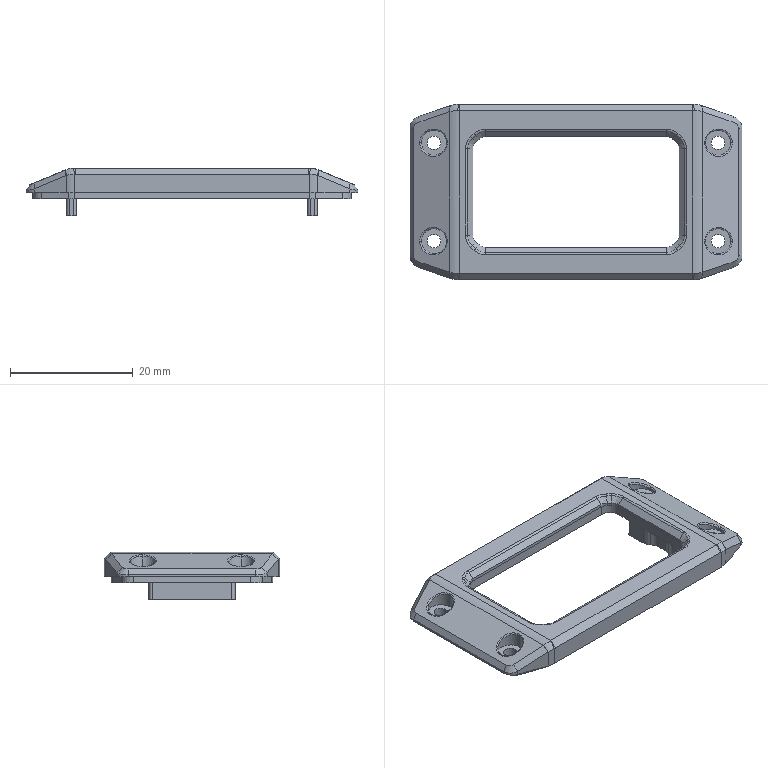Part | SolidWorks | features BaseBody 1 | 1 solid | 176 faces | box 54 x 28.5 x 7.8 mm | volume 2894 mm3 | cylinder 70 | plane 66 | spline 20 | cone 12 | torus 8 | commonest cylinder face diameters 4 x20 1 x16 2.2 x8 3 x8 4.1 x8 8 x6